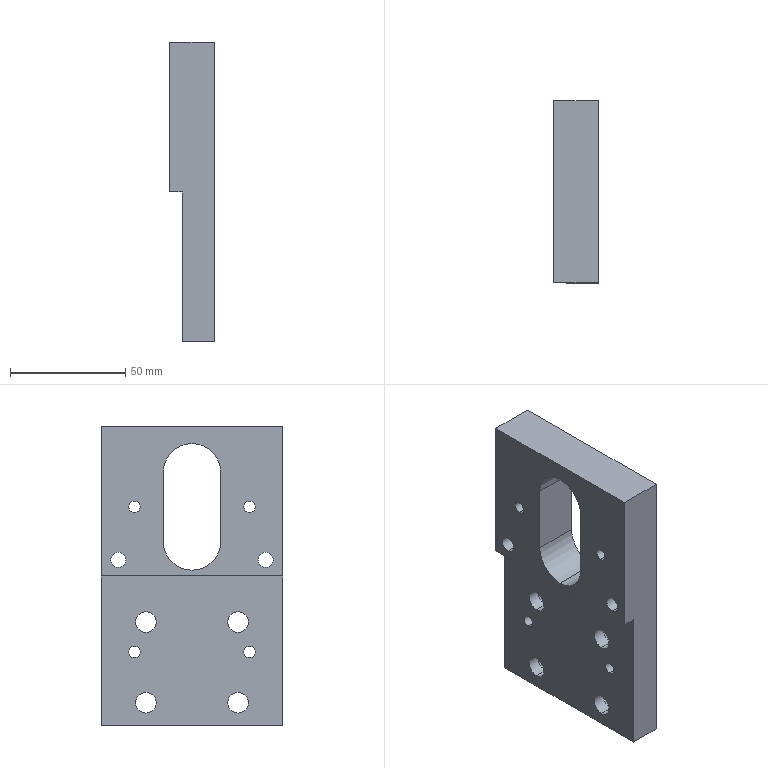Part | STEP file | PN_0010 (connecting plate) | 1 solid | 51 faces | box 19.5 x 79 x 130 mm | volume 136895 mm3 | cylinder 35 | plane 16 | commonest cylinder face diameters 5 x8 9 x8 15 x8 6.6 x4 11 x4 25 x3